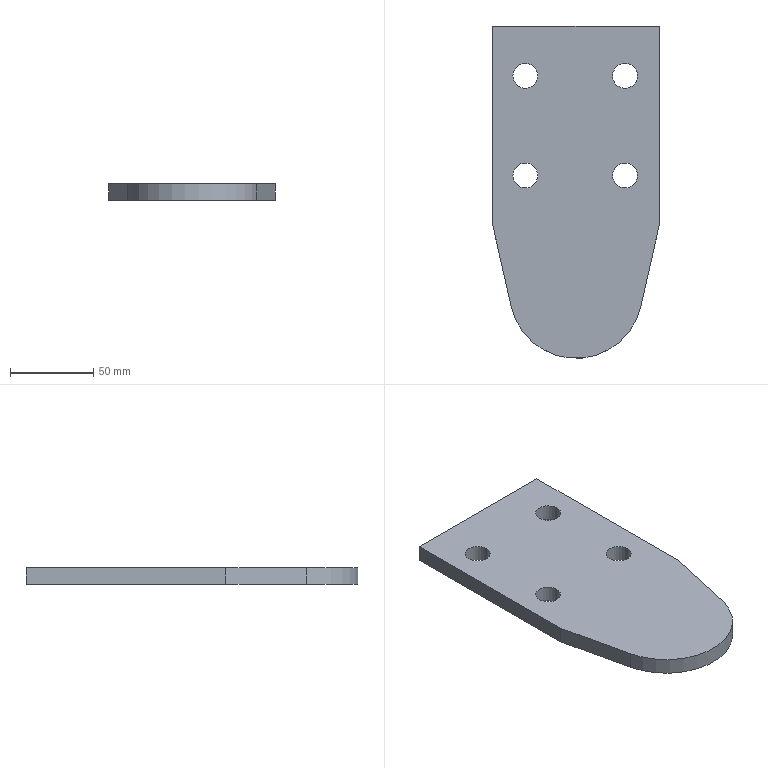Part | SolidWorks | features ICE 4, Extrusion 1 | 1 solid | 16 faces | box 100 x 200 x 10 mm | volume 174555 mm3 | cylinder 9 | plane 7 | commonest cylinder face diameters 15 x8 80 x1
STEP:
#1=CARTESIAN_POINT('',(7.033,-90.,0.));
#2=VERTEX_POINT('',#1);
#3=CARTESIAN_POINT('',(22.033,-90.,0.));
#4=VERTEX_POINT('',#3);
#5=CARTESIAN_POINT('',(14.533,-90.,0.));
#6=DIRECTION('',(0.,0.,1.));
#7=DIRECTION('',(1.,0.,0.));
#8=AXIS2_PLACEMENT_3D('',#5,#6,#7);
#9=CIRCLE('',#8,7.5);
#10=EDGE_CURVE('',#2,#4,#9,.T.);
#11=ORIENTED_EDGE('',*,*,#10,.F.);
#12=CARTESIAN_POINT('',(7.033,-90.,10.));
#13=VERTEX_POINT('',#12);
#14=CARTESIAN_POINT('',(7.033,-90.,0.));
#15=DIRECTION('',(0.,0.,1.));
#16=VECTOR('',#15,1000.);
#17=LINE('',#14,#16);
#18=EDGE_CURVE('',#2,#13,#17,.T.);
#19=ORIENTED_EDGE('',*,*,#18,.T.);
#20=CARTESIAN_POINT('',(22.033,-90.,10.));
#21=VERTEX_POINT('',#20);
#22=CARTESIAN_POINT('',(14.533,-90.,10.));
#23=DIRECTION('',(0.,0.,1.));
#24=DIRECTION('',(1.,0.,0.));
#25=AXIS2_PLACEMENT_3D('',#22,#23,#24);
#26=CIRCLE('',#25,7.5);
#27=EDGE_CURVE('',#13,#21,#26,.T.);
#28=ORIENTED_EDGE('',*,*,#27,.T.);
#29=CARTESIAN_POINT('',(22.033,-90.,0.));
#30=DIRECTION('',(0.,0.,1.));
#31=VECTOR('',#30,1000.);
#32=LINE('',#29,#31);
#33=EDGE_CURVE('',#4,#21,#32,.T.);
#34=ORIENTED_EDGE('',*,*,#33,.F.);
#35=EDGE_LOOP('',(#11,#19,#28,#34));
#36=FACE_OUTER_BOUND('',#35,.T.);
#37=CARTESIAN_POINT('',(14.533,-90.,0.));
#38=DIRECTION('',(0.,0.,1.));
#39=DIRECTION('',(1.,0.,0.));
#40=AXIS2_PLACEMENT_3D('',#37,#38,#39);
#41=CYLINDRICAL_SURFACE('',#40,7.5);
#42=ADVANCED_FACE('',(#36),#41,.F.);
#43=CARTESIAN_POINT('',(67.033,-90.,0.));
#44=VERTEX_POINT('',#43);
#45=CARTESIAN_POINT('',(82.033,-90.,0.));
#46=VERTEX_POINT('',#45);
#47=CARTESIAN_POINT('',(74.533,-90.,0.));
#48=DIRECTION('',(0.,0.,1.));
#49=DIRECTION('',(1.,0.,0.));
#50=AXIS2_PLACEMENT_3D('',#47,#48,#49);
#51=CIRCLE('',#50,7.5);
#52=EDGE_CURVE('',#44,#46,#51,.T.);
#53=ORIENTED_EDGE('',*,*,#52,.F.);
#54=CARTESIAN_POINT('',(67.033,-90.,10.));
#55=VERTEX_POINT('',#54);
#56=CARTESIAN_POINT('',(67.033,-90.,0.));
#57=DIRECTION('',(0.,0.,1.));
#58=VECTOR('',#57,1000.);
#59=LINE('',#56,#58);
#60=EDGE_CURVE('',#44,#55,#59,.T.);
#61=ORIENTED_EDGE('',*,*,#60,.T.);
#62=CARTESIAN_POINT('',(82.033,-90.,10.));
#63=VERTEX_POINT('',#62);
#64=CARTESIAN_POINT('',(74.533,-90.,10.));
#65=DIRECTION('',(0.,0.,1.));
#66=DIRECTION('',(1.,0.,0.));
#67=AXIS2_PLACEMENT_3D('',#64,#65,#66);
#68=CIRCLE('',#67,7.5);
#69=EDGE_CURVE('',#55,#63,#68,.T.);
#70=ORIENTED_EDGE('',*,*,#69,.T.);
#71=CARTESIAN_POINT('',(82.033,-90.,0.));
#72=DIRECTION('',(0.,0.,1.));
#73=VECTOR('',#72,1000.);
#74=LINE('',#71,#73);
#75=EDGE_CURVE('',#46,#63,#74,.T.);
#76=ORIENTED_EDGE('',*,*,#75,.F.);
#77=EDGE_LOOP('',(#53,#61,#70,#76));
#78=FACE_OUTER_BOUND('',#77,.T.);
#79=CARTESIAN_POINT('',(74.533,-90.,0.));
#80=DIRECTION('',(0.,0.,1.));
#81=DIRECTION('',(1.,0.,0.));
#82=AXIS2_PLACEMENT_3D('',#79,#80,#81);
#83=CYLINDRICAL_SURFACE('',#82,7.5);
#84=ADVANCED_FACE('',(#78),#83,.F.);
#85=CARTESIAN_POINT('',(67.033,-30.,0.));
#86=VERTEX_POINT('',#85);
#87=CARTESIAN_POINT('',(82.033,-30.,0.));
#88=VERTEX_POINT('',#87);
#89=CARTESIAN_POINT('',(74.533,-30.,0.));
#90=DIRECTION('',(0.,0.,1.));
#91=DIRECTION('',(1.,0.,0.));
#92=AXIS2_PLACEMENT_3D('',#89,#90,#91);
#93=CIRCLE('',#92,7.5);
#94=EDGE_CURVE('',#86,#88,#93,.T.);
#95=ORIENTED_EDGE('',*,*,#94,.F.);
#96=CARTESIAN_POINT('',(67.033,-30.,10.));
#97=VERTEX_POINT('',#96);
#98=CARTESIAN_POINT('',(67.033,-30.,0.));
#99=DIRECTION('',(0.,0.,1.));
#100=VECTOR('',#99,1000.);
#101=LINE('',#98,#100);
#102=EDGE_CURVE('',#86,#97,#101,.T.);
#103=ORIENTED_EDGE('',*,*,#102,.T.);
#104=CARTESIAN_POINT('',(82.033,-30.,10.));
#105=VERTEX_POINT('',#104);
#106=CARTESIAN_POINT('',(74.533,-30.,10.));
#107=DIRECTION('',(0.,0.,1.));
#108=DIRECTION('',(1.,0.,0.));
#109=AXIS2_PLACEMENT_3D('',#106,#107,#108);
#110=CIRCLE('',#109,7.5);
#111=EDGE_CURVE('',#97,#105,#110,.T.);
#112=ORIENTED_EDGE('',*,*,#111,.T.);
#113=CARTESIAN_POINT('',(82.033,-30.,0.));
#114=DIRECTION('',(0.,0.,1.));
#115=VECTOR('',#114,1000.);
#116=LINE('',#113,#115);
#117=EDGE_CURVE('',#88,#105,#116,.T.);
#118=ORIENTED_EDGE('',*,*,#117,.F.);
#119=EDGE_LOOP('',(#95,#103,#112,#118));
#120=FACE_OUTER_BOUND('',#119,.T.);
#121=CARTESIAN_POINT('',(74.533,-30.,0.));
#122=DIRECTION('',(0.,0.,1.));
#123=DIRECTION('',(1.,0.,0.));
#124=AXIS2_PLACEMENT_3D('',#121,#122,#123);
#125=CYLINDRICAL_SURFACE('',#124,7.5);
#126=ADVANCED_FACE('',(#120),#125,.F.);
#127=CARTESIAN_POINT('',(7.033,-30.,0.));
#128=VERTEX_POINT('',#127);
#129=CARTESIAN_POINT('',(22.033,-30.,0.));
#130=VERTEX_POINT('',#129);
#131=CARTESIAN_POINT('',(14.533,-30.,0.));
#132=DIRECTION('',(0.,0.,1.));
#133=DIRECTION('',(1.,0.,0.));
#134=AXIS2_PLACEMENT_3D('',#131,#132,#133);
#135=CIRCLE('',#134,7.5);
#136=EDGE_CURVE('',#128,#130,#135,.T.);
#137=ORIENTED_EDGE('',*,*,#136,.F.);
#138=CARTESIAN_POINT('',(7.033,-30.,10.));
#139=VERTEX_POINT('',#138);
#140=CARTESIAN_POINT('',(7.033,-30.,0.));
#141=DIRECTION('',(0.,0.,1.));
#142=VECTOR('',#141,1000.);
#143=LINE('',#140,#142);
#144=EDGE_CURVE('',#128,#139,#143,.T.);
#145=ORIENTED_EDGE('',*,*,#144,.T.);
#146=CARTESIAN_POINT('',(22.033,-30.,10.));
#147=VERTEX_POINT('',#146);
#148=CARTESIAN_POINT('',(14.533,-30.,10.));
#149=DIRECTION('',(0.,0.,1.));
#150=DIRECTION('',(1.,0.,0.));
#151=AXIS2_PLACEMENT_3D('',#148,#149,#150);
#152=CIRCLE('',#151,7.5);
#153=EDGE_CURVE('',#139,#147,#152,.T.);
#154=ORIENTED_EDGE('',*,*,#153,.T.);
#155=CARTESIAN_POINT('',(22.033,-30.,0.));
#156=DIRECTION('',(0.,0.,1.));
#157=VECTOR('',#156,1000.);
#158=LINE('',#155,#157);
#159=EDGE_CURVE('',#130,#147,#158,.T.);
#160=ORIENTED_EDGE('',*,*,#159,.F.);
#161=EDGE_LOOP('',(#137,#145,#154,#160));
#162=FACE_OUTER_BOUND('',#161,.T.);
#163=CARTESIAN_POINT('',(14.533,-30.,0.));
#164=DIRECTION('',(0.,0.,1.));
#165=DIRECTION('',(1.,0.,0.));
#166=AXIS2_PLACEMENT_3D('',#163,#164,#165);
#167=CYLINDRICAL_SURFACE('',#166,7.5);
#168=ADVANCED_FACE('',(#162),#167,.F.);
#169=CARTESIAN_POINT('',(5.987,-168.831,10.));
#170=VERTEX_POINT('',#169);
#171=CARTESIAN_POINT('',(84.013,-168.831,10.));
#172=VERTEX_POINT('',#171);
#173=CARTESIAN_POINT('',(45.,-160.,10.));
#174=DIRECTION('',(0.,0.,1.));
#175=DIRECTION('',(1.,0.,0.));
#176=AXIS2_PLACEMENT_3D('',#173,#174,#175);
#177=CIRCLE('',#176,40.);
#178=EDGE_CURVE('',#170,#172,#177,.T.);
#179=ORIENTED_EDGE('',*,*,#178,.F.);
#180=CARTESIAN_POINT('',(5.987,-168.831,0.));
#181=VERTEX_POINT('',#180);
#182=CARTESIAN_POINT('',(5.987,-168.831,10.));
#183=DIRECTION('',(0.,0.,-1.));
#184=VECTOR('',#183,1000.);
#185=LINE('',#182,#184);
#186=EDGE_CURVE('',#170,#181,#185,.T.);
#187=ORIENTED_EDGE('',*,*,#186,.T.);
#188=CARTESIAN_POINT('',(84.013,-168.831,0.));
#189=VERTEX_POINT('',#188);
#190=CARTESIAN_POINT('',(45.,-160.,0.));
#191=DIRECTION('',(0.,0.,1.));
#192=DIRECTION('',(1.,0.,0.));
#193=AXIS2_PLACEMENT_3D('',#190,#191,#192);
#194=CIRCLE('',#193,40.);
#195=EDGE_CURVE('',#181,#189,#194,.T.);
#196=ORIENTED_EDGE('',*,*,#195,.T.);
#197=CARTESIAN_POINT('',(84.013,-168.831,10.));
#198=DIRECTION('',(0.,0.,-1.));
#199=VECTOR('',#198,1000.);
#200=LINE('',#197,#199);
#201=EDGE_CURVE('',#172,#189,#200,.T.);
#202=ORIENTED_EDGE('',*,*,#201,.F.);
#203=EDGE_LOOP('',(#179,#187,#196,#202));
#204=FACE_OUTER_BOUND('',#203,.T.);
#205=CARTESIAN_POINT('',(45.,-160.,10.));
#206=DIRECTION('',(0.,0.,-1.));
#207=DIRECTION('',(-1.,0.,0.));
#208=AXIS2_PLACEMENT_3D('',#205,#206,#207);
#209=CYLINDRICAL_SURFACE('',#208,40.);
#210=ADVANCED_FACE('',(#204),#209,.T.);
#211=CARTESIAN_POINT('',(-5.,-120.294,10.));
#212=VERTEX_POINT('',#211);
#213=CARTESIAN_POINT('',(-30.659,-6.94,10.));
#214=DIRECTION('',(0.2208,-0.9753,0.));
#215=VECTOR('',#214,1000.);
#216=LINE('',#213,#215);
#217=EDGE_CURVE('',#212,#170,#216,.T.);
#218=ORIENTED_EDGE('',*,*,#217,.T.);
#219=ORIENTED_EDGE('',*,*,#178,.T.);
#220=CARTESIAN_POINT('',(95.,-120.294,10.));
#221=VERTEX_POINT('',#220);
#222=CARTESIAN_POINT('',(116.272,-26.32,10.));
#223=DIRECTION('',(-0.2208,-0.9753,0.));
#224=VECTOR('',#223,1000.);
#225=LINE('',#222,#224);
#226=EDGE_CURVE('',#221,#172,#225,.T.);
#227=ORIENTED_EDGE('',*,*,#226,.F.);
#228=CARTESIAN_POINT('',(95.,0.,10.));
#229=VERTEX_POINT('',#228);
#230=CARTESIAN_POINT('',(95.,0.,10.));
#231=DIRECTION('',(0.,-1.,0.));
#232=VECTOR('',#231,1000.);
#233=LINE('',#230,#232);
#234=EDGE_CURVE('',#229,#221,#233,.T.);
#235=ORIENTED_EDGE('',*,*,#234,.F.);
#236=CARTESIAN_POINT('',(-5.,0.,10.));
#237=VERTEX_POINT('',#236);
#238=CARTESIAN_POINT('',(0.,0.,10.));
#239=DIRECTION('',(-1.,0.,0.));
#240=VECTOR('',#239,1000.);
#241=LINE('',#238,#240);
#242=EDGE_CURVE('',#229,#237,#241,.T.);
#243=ORIENTED_EDGE('',*,*,#242,.T.);
#244=CARTESIAN_POINT('',(-5.,0.,10.));
#245=DIRECTION('',(0.,-1.,0.));
#246=VECTOR('',#245,1000.);
#247=LINE('',#244,#246);
#248=EDGE_CURVE('',#237,#212,#247,.T.);
#249=ORIENTED_EDGE('',*,*,#248,.T.);
#250=EDGE_LOOP('',(#218,#219,#227,#235,#243,#249));
#251=FACE_OUTER_BOUND('',#250,.T.);
#252=CARTESIAN_POINT('',(14.533,-90.,10.));
#253=DIRECTION('',(0.,0.,1.));
#254=DIRECTION('',(1.,0.,0.));
#255=AXIS2_PLACEMENT_3D('',#252,#253,#254);
#256=CIRCLE('',#255,7.5);
#257=EDGE_CURVE('',#21,#13,#256,.T.);
#258=ORIENTED_EDGE('',*,*,#257,.F.);
#259=ORIENTED_EDGE('',*,*,#27,.F.);
#260=EDGE_LOOP('',(#258,#259));
#261=FACE_BOUND('',#260,.T.);
#262=CARTESIAN_POINT('',(74.533,-90.,10.));
#263=DIRECTION('',(0.,0.,1.));
#264=DIRECTION('',(1.,0.,0.));
#265=AXIS2_PLACEMENT_3D('',#262,#263,#264);
#266=CIRCLE('',#265,7.5);
#267=EDGE_CURVE('',#63,#55,#266,.T.);
#268=ORIENTED_EDGE('',*,*,#267,.F.);
#269=ORIENTED_EDGE('',*,*,#69,.F.);
#270=EDGE_LOOP('',(#268,#269));
#271=FACE_BOUND('',#270,.T.);
#272=CARTESIAN_POINT('',(74.533,-30.,10.));
#273=DIRECTION('',(0.,0.,1.));
#274=DIRECTION('',(1.,0.,0.));
#275=AXIS2_PLACEMENT_3D('',#272,#273,#274);
#276=CIRCLE('',#275,7.5);
#277=EDGE_CURVE('',#105,#97,#276,.T.);
#278=ORIENTED_EDGE('',*,*,#277,.F.);
#279=ORIENTED_EDGE('',*,*,#111,.F.);
#280=EDGE_LOOP('',(#278,#279));
#281=FACE_BOUND('',#280,.T.);
#282=CARTESIAN_POINT('',(14.533,-30.,10.));
#283=DIRECTION('',(0.,0.,1.));
#284=DIRECTION('',(1.,0.,0.));
#285=AXIS2_PLACEMENT_3D('',#282,#283,#284);
#286=CIRCLE('',#285,7.5);
#287=EDGE_CURVE('',#147,#139,#286,.T.);
#288=ORIENTED_EDGE('',*,*,#287,.F.);
#289=ORIENTED_EDGE('',*,*,#153,.F.);
#290=EDGE_LOOP('',(#288,#289));
#291=FACE_BOUND('',#290,.T.);
#292=CARTESIAN_POINT('',(45.,-160.,10.));
#293=DIRECTION('',(0.,0.,1.));
#294=DIRECTION('',(1.,0.,0.));
#295=AXIS2_PLACEMENT_3D('',#292,#293,#294);
#296=PLANE('',#295);
#297=ADVANCED_FACE('',(#251,#261,#271,#281,#291),#296,.T.);
#298=ORIENTED_EDGE('',*,*,#195,.F.);
#299=CARTESIAN_POINT('',(-5.,-120.294,0.));
#300=VERTEX_POINT('',#299);
#301=CARTESIAN_POINT('',(-30.659,-6.94,0.));
#302=DIRECTION('',(0.2208,-0.9753,0.));
#303=VECTOR('',#302,1000.);
#304=LINE('',#301,#303);
#305=EDGE_CURVE('',#300,#181,#304,.T.);
#306=ORIENTED_EDGE('',*,*,#305,.F.);
#307=CARTESIAN_POINT('',(-5.,0.,0.));
#308=VERTEX_POINT('',#307);
#309=CARTESIAN_POINT('',(-5.,0.,0.));
#310=DIRECTION('',(0.,-1.,0.));
#311=VECTOR('',#310,1000.);
#312=LINE('',#309,#311);
#313=EDGE_CURVE('',#308,#300,#312,.T.);
#314=ORIENTED_EDGE('',*,*,#313,.F.);
#315=CARTESIAN_POINT('',(95.,0.,0.));
#316=VERTEX_POINT('',#315);
#317=CARTESIAN_POINT('',(0.,0.,0.));
#318=DIRECTION('',(-1.,0.,0.));
#319=VECTOR('',#318,1000.);
#320=LINE('',#317,#319);
#321=EDGE_CURVE('',#316,#308,#320,.T.);
#322=ORIENTED_EDGE('',*,*,#321,.F.);
#323=CARTESIAN_POINT('',(95.,-120.294,0.));
#324=VERTEX_POINT('',#323);
#325=CARTESIAN_POINT('',(95.,0.,0.));
#326=DIRECTION('',(0.,-1.,0.));
#327=VECTOR('',#326,1000.);
#328=LINE('',#325,#327);
#329=EDGE_CURVE('',#316,#324,#328,.T.);
#330=ORIENTED_EDGE('',*,*,#329,.T.);
#331=CARTESIAN_POINT('',(116.272,-26.32,0.));
#332=DIRECTION('',(-0.2208,-0.9753,0.));
#333=VECTOR('',#332,1000.);
#334=LINE('',#331,#333);
#335=EDGE_CURVE('',#324,#189,#334,.T.);
#336=ORIENTED_EDGE('',*,*,#335,.T.);
#337=EDGE_LOOP('',(#298,#306,#314,#322,#330,#336));
#338=FACE_OUTER_BOUND('',#337,.T.);
#339=CARTESIAN_POINT('',(14.533,-90.,0.));
#340=DIRECTION('',(0.,0.,1.));
#341=DIRECTION('',(1.,0.,0.));
#342=AXIS2_PLACEMENT_3D('',#339,#340,#341);
#343=CIRCLE('',#342,7.5);
#344=EDGE_CURVE('',#4,#2,#343,.T.);
#345=ORIENTED_EDGE('',*,*,#344,.T.);
#346=ORIENTED_EDGE('',*,*,#10,.T.);
#347=EDGE_LOOP('',(#345,#346));
#348=FACE_BOUND('',#347,.T.);
#349=CARTESIAN_POINT('',(74.533,-90.,0.));
#350=DIRECTION('',(0.,0.,1.));
#351=DIRECTION('',(1.,0.,0.));
#352=AXIS2_PLACEMENT_3D('',#349,#350,#351);
#353=CIRCLE('',#352,7.5);
#354=EDGE_CURVE('',#46,#44,#353,.T.);
#355=ORIENTED_EDGE('',*,*,#354,.T.);
#356=ORIENTED_EDGE('',*,*,#52,.T.);
#357=EDGE_LOOP('',(#355,#356));
#358=FACE_BOUND('',#357,.T.);
#359=CARTESIAN_POINT('',(74.533,-30.,0.));
#360=DIRECTION('',(0.,0.,1.));
#361=DIRECTION('',(1.,0.,0.));
#362=AXIS2_PLACEMENT_3D('',#359,#360,#361);
#363=CIRCLE('',#362,7.5);
#364=EDGE_CURVE('',#88,#86,#363,.T.);
#365=ORIENTED_EDGE('',*,*,#364,.T.);
#366=ORIENTED_EDGE('',*,*,#94,.T.);
#367=EDGE_LOOP('',(#365,#366));
#368=FACE_BOUND('',#367,.T.);
#369=CARTESIAN_POINT('',(14.533,-30.,0.));
#370=DIRECTION('',(0.,0.,1.));
#371=DIRECTION('',(1.,0.,0.));
#372=AXIS2_PLACEMENT_3D('',#369,#370,#371);
#373=CIRCLE('',#372,7.5);
#374=EDGE_CURVE('',#130,#128,#373,.T.);
#375=ORIENTED_EDGE('',*,*,#374,.T.);
#376=ORIENTED_EDGE('',*,*,#136,.T.);
#377=EDGE_LOOP('',(#375,#376));
#378=FACE_BOUND('',#377,.T.);
#379=CARTESIAN_POINT('',(45.,-160.,0.));
#380=DIRECTION('',(0.,0.,1.));
#381=DIRECTION('',(1.,0.,0.));
#382=AXIS2_PLACEMENT_3D('',#379,#380,#381);
#383=PLANE('',#382);
#384=ADVANCED_FACE('',(#338,#348,#358,#368,#378),#383,.F.);
#385=ORIENTED_EDGE('',*,*,#321,.T.);
#386=CARTESIAN_POINT('',(-5.,0.,10.));
#387=DIRECTION('',(0.,0.,-1.));
#388=VECTOR('',#387,1000.);
#389=LINE('',#386,#388);
#390=EDGE_CURVE('',#237,#308,#389,.T.);
#391=ORIENTED_EDGE('',*,*,#390,.F.);
#392=ORIENTED_EDGE('',*,*,#242,.F.);
#393=CARTESIAN_POINT('',(95.,0.,10.));
#394=DIRECTION('',(0.,0.,-1.));
#395=VECTOR('',#394,1000.);
#396=LINE('',#393,#395);
#397=EDGE_CURVE('',#229,#316,#396,.T.);
#398=ORIENTED_EDGE('',*,*,#397,.T.);
#399=EDGE_LOOP('',(#385,#391,#392,#398));
#400=FACE_OUTER_BOUND('',#399,.T.);
#401=CARTESIAN_POINT('',(0.,0.,10.));
#402=DIRECTION('',(0.,-1.,0.));
#403=DIRECTION('',(0.,0.,-1.));
#404=AXIS2_PLACEMENT_3D('',#401,#402,#403);
#405=PLANE('',#404);
#406=ADVANCED_FACE('',(#400),#405,.F.);
#407=ORIENTED_EDGE('',*,*,#144,.F.);
#408=ORIENTED_EDGE('',*,*,#374,.F.);
#409=ORIENTED_EDGE('',*,*,#159,.T.);
#410=ORIENTED_EDGE('',*,*,#287,.T.);
#411=EDGE_LOOP('',(#407,#408,#409,#410));
#412=FACE_OUTER_BOUND('',#411,.T.);
#413=CARTESIAN_POINT('',(14.533,-30.,0.));
#414=DIRECTION('',(0.,0.,1.));
#415=DIRECTION('',(1.,0.,0.));
#416=AXIS2_PLACEMENT_3D('',#413,#414,#415);
#417=CYLINDRICAL_SURFACE('',#416,7.5);
#418=ADVANCED_FACE('',(#412),#417,.F.);
#419=ORIENTED_EDGE('',*,*,#102,.F.);
#420=ORIENTED_EDGE('',*,*,#364,.F.);
#421=ORIENTED_EDGE('',*,*,#117,.T.);
#422=ORIENTED_EDGE('',*,*,#277,.T.);
#423=EDGE_LOOP('',(#419,#420,#421,#422));
#424=FACE_OUTER_BOUND('',#423,.T.);
#425=CARTESIAN_POINT('',(74.533,-30.,0.));
#426=DIRECTION('',(0.,0.,1.));
#427=DIRECTION('',(1.,0.,0.));
#428=AXIS2_PLACEMENT_3D('',#425,#426,#427);
#429=CYLINDRICAL_SURFACE('',#428,7.5);
#430=ADVANCED_FACE('',(#424),#429,.F.);
#431=ORIENTED_EDGE('',*,*,#60,.F.);
#432=ORIENTED_EDGE('',*,*,#354,.F.);
#433=ORIENTED_EDGE('',*,*,#75,.T.);
#434=ORIENTED_EDGE('',*,*,#267,.T.);
#435=EDGE_LOOP('',(#431,#432,#433,#434));
#436=FACE_OUTER_BOUND('',#435,.T.);
#437=CARTESIAN_POINT('',(74.533,-90.,0.));
#438=DIRECTION('',(0.,0.,1.));
#439=DIRECTION('',(1.,0.,0.));
#440=AXIS2_PLACEMENT_3D('',#437,#438,#439);
#441=CYLINDRICAL_SURFACE('',#440,7.5);
#442=ADVANCED_FACE('',(#436),#441,.F.);
#443=ORIENTED_EDGE('',*,*,#18,.F.);
#444=ORIENTED_EDGE('',*,*,#344,.F.);
#445=ORIENTED_EDGE('',*,*,#33,.T.);
#446=ORIENTED_EDGE('',*,*,#257,.T.);
#447=EDGE_LOOP('',(#443,#444,#445,#446));
#448=FACE_OUTER_BOUND('',#447,.T.);
#449=CARTESIAN_POINT('',(14.533,-90.,0.));
#450=DIRECTION('',(0.,0.,1.));
#451=DIRECTION('',(1.,0.,0.));
#452=AXIS2_PLACEMENT_3D('',#449,#450,#451);
#453=CYLINDRICAL_SURFACE('',#452,7.5);
#454=ADVANCED_FACE('',(#448),#453,.F.);
#455=ORIENTED_EDGE('',*,*,#329,.F.);
#456=ORIENTED_EDGE('',*,*,#397,.F.);
#457=ORIENTED_EDGE('',*,*,#234,.T.);
#458=CARTESIAN_POINT('',(95.,-120.294,10.));
#459=DIRECTION('',(0.,0.,-1.));
#460=VECTOR('',#459,1000.);
#461=LINE('',#458,#460);
#462=EDGE_CURVE('',#221,#324,#461,.T.);
#463=ORIENTED_EDGE('',*,*,#462,.T.);
#464=EDGE_LOOP('',(#455,#456,#457,#463));
#465=FACE_OUTER_BOUND('',#464,.T.);
#466=CARTESIAN_POINT('',(95.,0.,10.));
#467=DIRECTION('',(1.,0.,0.));
#468=DIRECTION('',(0.,1.,0.));
#469=AXIS2_PLACEMENT_3D('',#466,#467,#468);
#470=PLANE('',#469);
#471=ADVANCED_FACE('',(#465),#470,.T.);
#472=ORIENTED_EDGE('',*,*,#335,.F.);
#473=ORIENTED_EDGE('',*,*,#462,.F.);
#474=ORIENTED_EDGE('',*,*,#226,.T.);
#475=ORIENTED_EDGE('',*,*,#201,.T.);
#476=EDGE_LOOP('',(#472,#473,#474,#475));
#477=FACE_OUTER_BOUND('',#476,.T.);
#478=CARTESIAN_POINT('',(116.272,-26.32,10.));
#479=DIRECTION('',(0.9753,-0.2208,0.));
#480=DIRECTION('',(0.2208,0.9753,0.));
#481=AXIS2_PLACEMENT_3D('',#478,#479,#480);
#482=PLANE('',#481);
#483=ADVANCED_FACE('',(#477),#482,.T.);
#484=ORIENTED_EDGE('',*,*,#305,.T.);
#485=ORIENTED_EDGE('',*,*,#186,.F.);
#486=ORIENTED_EDGE('',*,*,#217,.F.);
#487=CARTESIAN_POINT('',(-5.,-120.294,10.));
#488=DIRECTION('',(0.,0.,-1.));
#489=VECTOR('',#488,1000.);
#490=LINE('',#487,#489);
#491=EDGE_CURVE('',#212,#300,#490,.T.);
#492=ORIENTED_EDGE('',*,*,#491,.T.);
#493=EDGE_LOOP('',(#484,#485,#486,#492));
#494=FACE_OUTER_BOUND('',#493,.T.);
#495=CARTESIAN_POINT('',(-30.659,-6.94,10.));
#496=DIRECTION('',(0.9753,0.2208,0.));
#497=DIRECTION('',(-0.2208,0.9753,0.));
#498=AXIS2_PLACEMENT_3D('',#495,#496,#497);
#499=PLANE('',#498);
#500=ADVANCED_FACE('',(#494),#499,.F.);
#501=ORIENTED_EDGE('',*,*,#313,.T.);
#502=ORIENTED_EDGE('',*,*,#491,.F.);
#503=ORIENTED_EDGE('',*,*,#248,.F.);
#504=ORIENTED_EDGE('',*,*,#390,.T.);
#505=EDGE_LOOP('',(#501,#502,#503,#504));
#506=FACE_OUTER_BOUND('',#505,.T.);
#507=CARTESIAN_POINT('',(-5.,0.,10.));
#508=DIRECTION('',(1.,0.,0.));
#509=DIRECTION('',(0.,1.,0.));
#510=AXIS2_PLACEMENT_3D('',#507,#508,#509);
#511=PLANE('',#510);
#512=ADVANCED_FACE('',(#506),#511,.F.);
#513=CLOSED_SHELL('',(#42,#84,#126,#168,#210,#297,#384,#406,#418,#430,#442,#454,#471,#483,#500,#512));
#514=MANIFOLD_SOLID_BREP('',#513);
#515=CARTESIAN_POINT('',(0.,0.,0.));
#516=DIRECTION('',(0.,0.,1.));
#517=DIRECTION('',(1.,0.,0.));
#518=AXIS2_PLACEMENT_3D('',#515,#516,#517);
#519=(LENGTH_UNIT()NAMED_UNIT(*)SI_UNIT(.MILLI.,.METRE.));
#520=UNCERTAINTY_MEASURE_WITH_UNIT(LENGTH_MEASURE(0.00001),#519,'','');
#521=(NAMED_UNIT(*)PLANE_ANGLE_UNIT()SI_UNIT($,.RADIAN.));
#522=(NAMED_UNIT(*)SI_UNIT($,.STERADIAN.)SOLID_ANGLE_UNIT());
#523=(GEOMETRIC_REPRESENTATION_CONTEXT(3)GLOBAL_UNCERTAINTY_ASSIGNED_CONTEXT((#520))GLOBAL_UNIT_ASSIGNED_CONTEXT((#519,#521,#522))REPRESENTATION_CONTEXT('',''));
#524=ADVANCED_BREP_SHAPE_REPRESENTATION('',(#514,#518),#523);